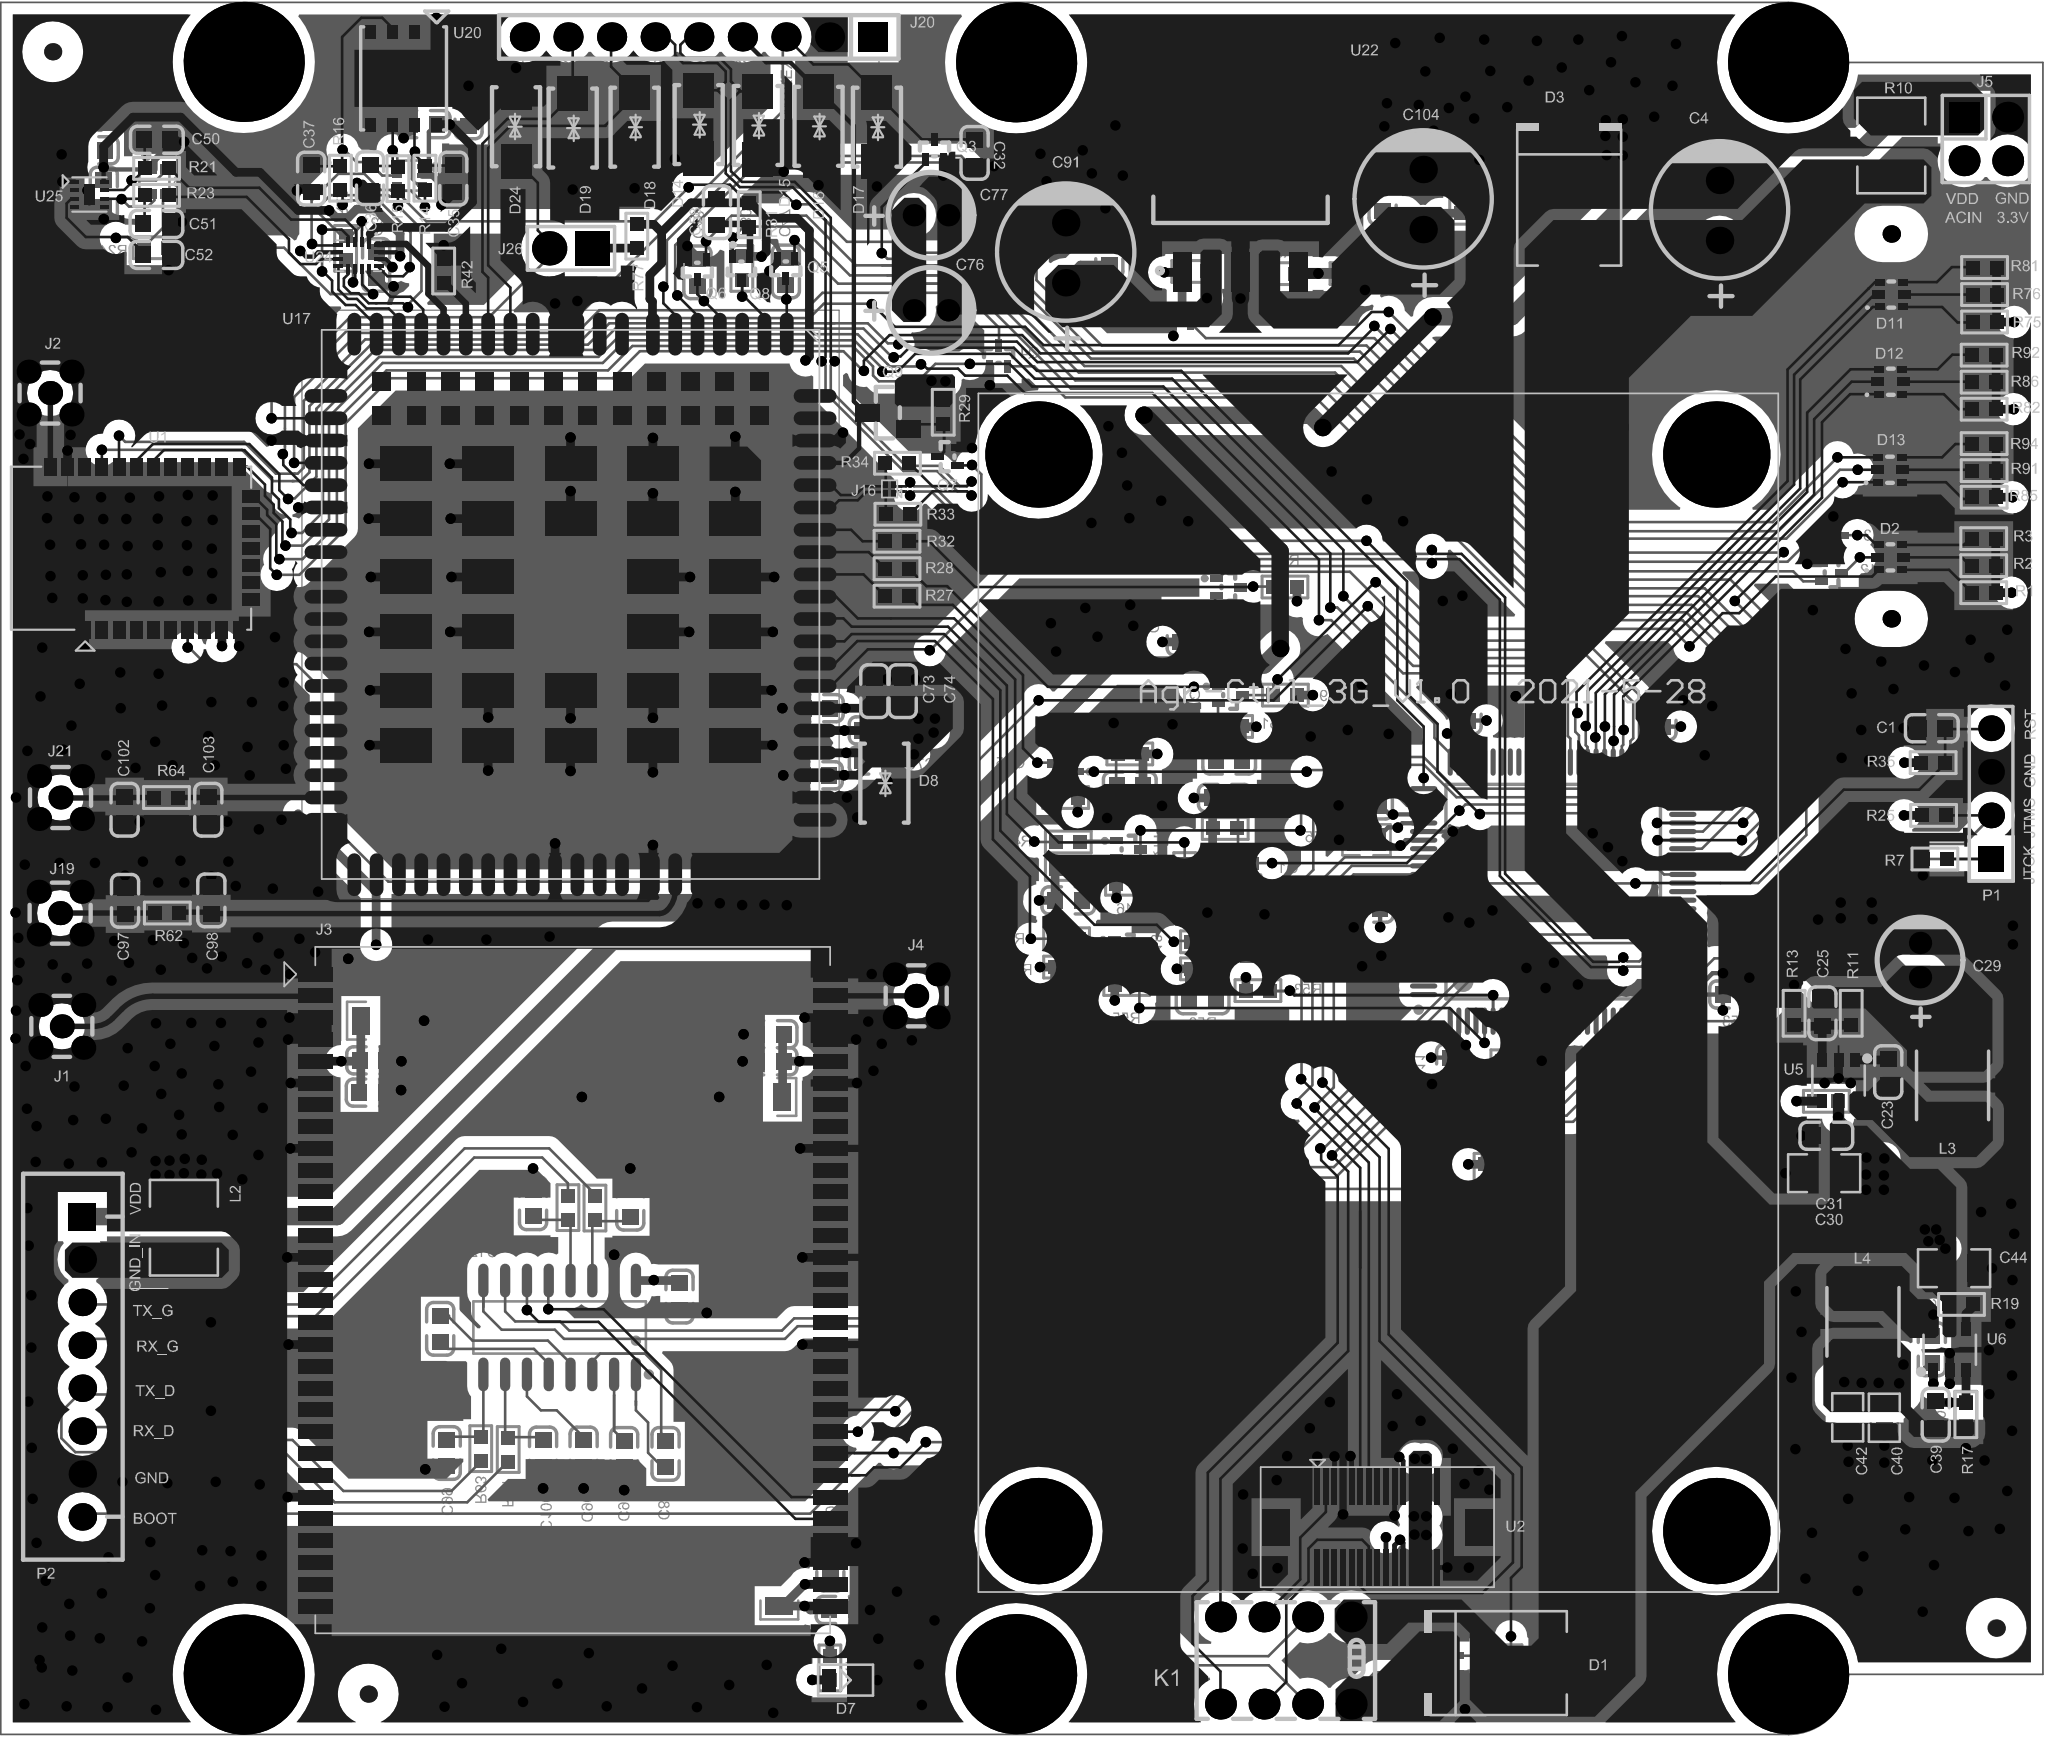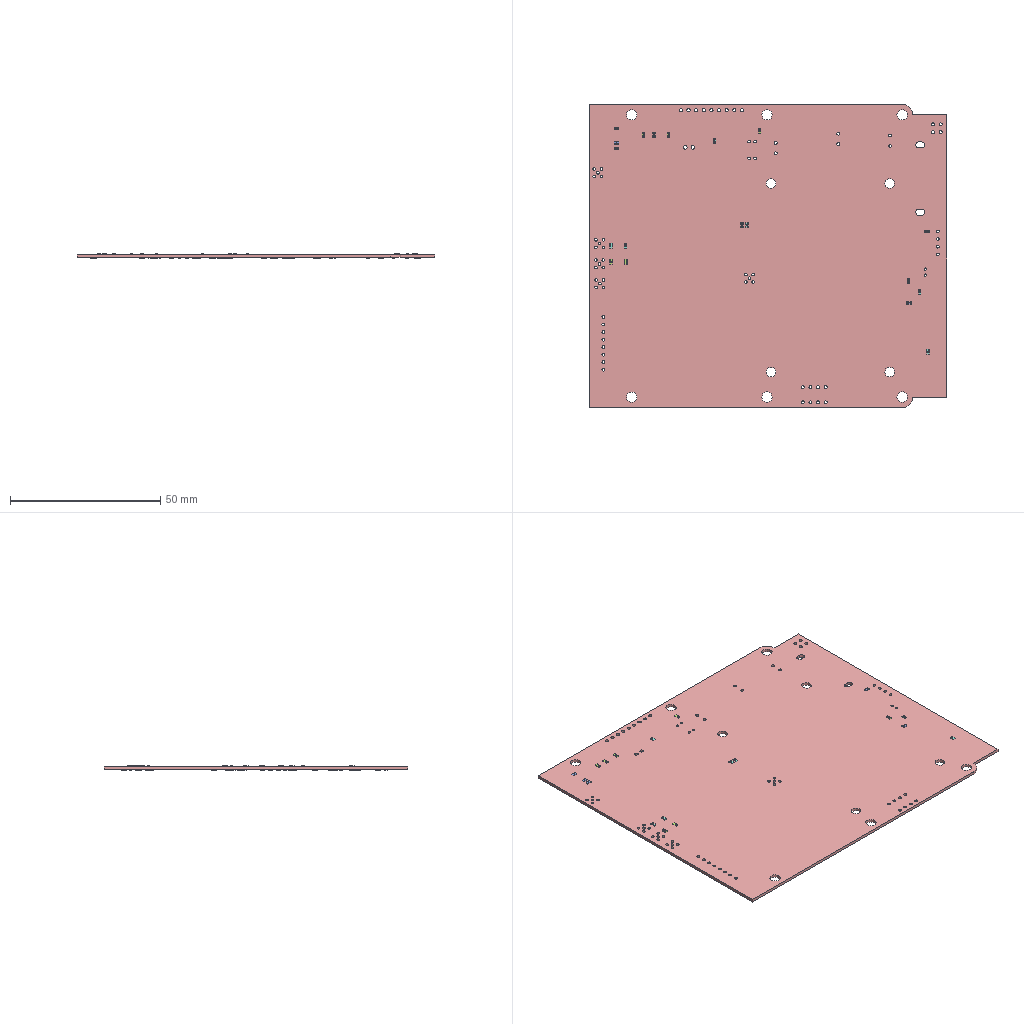Circuit board layout | Altium Designer | box 119 x 100.9 x 1.6 mm
Layer stack:
# Altium Designer layer stack of  (unit mm; dielectric type: 0 none, 1 core, 2 prepreg, 3 surface material)
index,name,kind,layer,copper_thickness_mm,dielectric_type,dielectric_thickness_mm,dielectric_material,dielectric_constant
0,Top Paste,other,,,,,,
1,Top Overlay,other,,,,,,
2,Top Solder,dielectric,,,3,0.0102,Solder Resist,3.5
3,TOP,copper,TOP,0.0305,,,,
4,Dielectric1,dielectric,,,1,0.2032,FR-4,4.5
5,GND,copper,GND,0.0356,,,,
6,Dielectric5,dielectric,,,2,0.32,FR-4,4.8
7,POWER,copper,POWER,0.0356,,,,
8,Dielectric6,dielectric,,,1,0.32,FR-4,4.8
9,BOTTOM,copper,BOTTOM,0.0305,,,,
10,Bottom Solder,dielectric,,,3,0.0102,Solder Resist,3.5
11,Bottom Overlay,other,,,,,,
12,Bottom Paste,other,,,,,,
# drill layer pairs: low layer,high layer
drill_pair,TOP,BOTTOM
Part placement:
Designator,Comment,Layer,Footprint,Center-X(mm),Center-Y(mm),Rotation
Q19,2SC4617TLQ,BottomLayer,SOT-416F_L1.6-W0.8-P1.00-LS1.6-TR,23.546,-26.391,270
Q18,2SC4617TLQ,BottomLayer,SOT-416F_L1.6-W0.8-P1.00-LS1.6-TR,4.953,15.342,90
Q17,2SC4617TLQ,BottomLayer,SOT-416F_L1.6-W0.8-P1.00-LS1.6-TR,12.624,15.215,90
Q16,2SC4617TLQ,BottomLayer,SOT-416F_L1.6-W0.8-P1.00-LS1.6-TR,10.973,30.099,90
Q15,2SC4617TLQ,BottomLayer,SOT-416F_L1.6-W0.8-P1.00-LS1.6-TR,1.397,26.137,270
Q14,2SC4617TLQ,BottomLayer,SOT-416F_L1.6-W0.8-P1.00-LS1.6-TR,5.055,21.107,90
C1,100nF/50V,TopLayer,C0603,51.867,28.169,360
C2,100nF/50V,BottomLayer,C0603,24.816,29.388,90
C3,100nF/50V,BottomLayer,C0603,36.17,29.032,90
C4,470uF/25V,TopLayer,RB8*11.5,39.497,58.344,90
C5,10uF/25V±10%,BottomLayer,C1206,-16.408,6.68,0
C6,100nF/50V,BottomLayer,C0603,-15.802,8.757,180
C7,100pF,BottomLayer,C0603,-15.799,10.338,180
C8,100pF,BottomLayer,C0603,-38.989,6.934,180
C9,100nF/50V,BottomLayer,C0603,-38.964,8.814,180
C10,10uF/25V±10%,BottomLayer,C1206,-38.379,11.125,180
C11,100nF/50V,BottomLayer,C0603,23.8,8.204,270
C20,100pF,BottomLayer,C0603,-12.319,-20.574,270
C21,100nF/50V,BottomLayer,C0603,-11.608,-23.216,180
C22,10uF/25V±10%,BottomLayer,C1206,-15.291,-21.666,270
C23,100nF/50V,TopLayer,C0603,49.327,8.128,90
C24,100nF/50V,BottomLayer,C0603,-33.401,64.059,90
C25,100pF,TopLayer,C0603,45.491,11.557,270
C26,22uF/10V±20%,BottomLayer,C0805,48.616,15.189,90
C27,100nF/50V,BottomLayer,C0603,44.577,15.189,90
C28,22uF/10V±20%,BottomLayer,C0805,46.558,15.189,90
C29,100uF/10V,TopLayer,RB5*7,51.181,14.656,90
C30,10uF/25V±10%,TopLayer,C1206,45.593,2.235,360
C31,100nF/50V,TopLayer,C0603,45.72,4.42,360
C32,10nF/50V,TopLayer,C0603,-3.912,61.697,270
C33,100nF/50V,BottomLayer,C0603,51.867,-8.026,270
C34,33pF/50V,BottomLayer,C0603,-36.017,63.373,180
C35,33pF/50V,TopLayer,C0603,-34.29,60.198,270
C36,33pF/50V,TopLayer,C0603,-39.141,60.223,270
C37,33pF/50V,TopLayer,C0603,-42.57,60.198,270
C38,100nF/50V,BottomLayer,C0603,-38.786,55.169,90
C39,100pF,TopLayer,C0603,52.095,-11.836,90
C40,22uF/10V±20%,TopLayer,C0805,49.098,-12.014,270
C41,100nF/50V,BottomLayer,C0603,49.098,-11.963,270
C42,22uF/10V±20%,TopLayer,C0805,46.965,-11.989,270
C43,22uF/10V±20%,BottomLayer,C0805,46.965,-11.989,270
C44,10uF/25V±10%,TopLayer,C1206,53.162,-3.302,180
C45,100nF/50V,BottomLayer,C0603,-55.347,61.849,180
C46,100nF/50V,BottomLayer,C0603,52.883,-0.0254,180
C47,10nF/50V,BottomLayer,C0603,-14.91,54.788,90
C48,10nF/50V,BottomLayer,C0603,-20.066,54.737,90
C49,33pF/50V,BottomLayer,C0603,-54.653,59.323,270
C50,33pF/50V,TopLayer,C0603,-51.562,62.459,360
C51,33pF/50V,TopLayer,C0603,-51.587,57.556,360
C52,33pF/50V,TopLayer,C0603,-51.587,55.753,360
C53,100nF/50V,BottomLayer,C0603,40.462,12.649,360
C54,100nF/50V,BottomLayer,C0603,18.948,17.653,180
C55,10nF/50V,BottomLayer,C0805,18.923,21.666,360
C56,100nF/50V,BottomLayer,C0603,18.898,23.673,180
C57,1nF/50V,BottomLayer,C0603,10.668,24.105,360
C58,1nF/50V,TopLayer,C0603,-18.923,58.242,90
C61,1nF/50V,BottomLayer,C0603,1.549,18.136,180
C62,1nF/50V,BottomLayer,C0603,10.922,26.289,360
C70,100nF/50V,BottomLayer,C0603,-9.677,26.289,360
C71,33pF/50V,BottomLayer,C0603,-9.677,28.042,360
C72,12pF/50V,BottomLayer,C0603,-13.106,29.337,180
C73,100nF/50V,TopLayer,C0603,-9.754,30.328,90
C74,33pF/50V,TopLayer,C0603,-8.103,30.328,90
C75,12pF/50V,BottomLayer,C0603,-13.157,25.425,180
C76,100uF/10V,TopLayer,RB5*7,-6.452,52.527,360
C77,100uF/10V,TopLayer,RB5*7,-6.452,58.064,360
C91,470uF/25V,TopLayer,RB8*11.5,1.397,55.88,90
C97,NM,TopLayer,C0603,-53.416,18.11,270
C98,NM,TopLayer,C0603,-48.387,18.136,270
C101,100nF/50V,BottomLayer,C0603,3.937,55.931,90
C102,NM,TopLayer,C0603,-53.442,23.419,90
C103,NM,TopLayer,C0603,-48.565,23.419,90
C104,470uF/25V,TopLayer,RB8*11.5,22.225,58.979,90
C105,100nF/50V,BottomLayer,C0603,19.863,59.055,90
D1,SMCJ18A,TopLayer,SMC,26.619,-26.314,360
D2,RGB,TopLayer,RGB,49.454,38.125,180
D3,SMCJ18A,TopLayer,SMC,30.734,59.106,270
D7,GREEN,TopLayer,LED0805,-11.43,-27.305,360
D8,SMAJ6.8CA,TopLayer,SMA,-9.169,24.968,180
D11,RGB,TopLayer,RGB,49.505,53.442,180
D12,RGB,TopLayer,RGB,49.479,48.362,180
D13,RGB,TopLayer,RGB,49.428,43.231,180
D14,SMAJ6.8CA,TopLayer,SMA,-19.99,63.348,180
D15,SMAJ6.8CA,TopLayer,SMA,-16.535,63.297,180
D16,SMAJ6.8CA,TopLayer,SMA,-13.005,63.246,180
D17,SMAJ6.8CA,TopLayer,SMA,-9.601,63.195,180
D18,SMAJ6.8CA,TopLayer,SMA,-23.724,63.195,180
D19,SMAJ6.8CA,TopLayer,SMA,-27.33,63.144,180
D24,SMAJ6.8CA,TopLayer,SMA,-30.632,63.221,360
J3,UM482/K823,TopLayer,UM482/K823,-27.33,-4.572,360
J4,MMCX-KE RF connector,TopLayer,MMCX-KE,-7.315,12.573,0
J5,POWER,TopLayer,2.54mm_2x2,55.016,62.509,270
U20,SIM-A China Telecom eSIM,TopLayer,VQFN8,-37.186,66.04,270
U23,ESDA6V8V6-6,BottomLayer,SOT-563,-36.83,60.376,180
U24,FSA2567MPX,TopLayer,MLP-16,-39.802,55.702,180
U25,SIM-B China Mobile eSIM,TopLayer,DFN2*2-8,-55.491,59.272,0
U26,ESDA6V8V6-6,BottomLayer,SOT-563,-51.706,60.009,270
J16,DLM0NSN900HY2D,TopLayer,SMD_0.85x0.65mm,-8.865,42.113,180
J20,2.54_9,TopLayer,2.54-9P,-19.984,68.456,180
J21,MMCX-KE RF connector,TopLayer,MMCX-KE,-57.175,24.13,0
L2,120Ω ±25% @100MHz,TopLayer,1812,-49.987,-0.9398,90
L3,2.2uH/2A,TopLayer,SMD,4x4x2.6mm,53.075,7.354,90
L4,2.2uH/2A,TopLayer,SMD,4x4x2.6mm,47.854,-6.426,270
P1,Header 4,TopLayer,HDR1X4,55.321,24.359,90
P2,XH-8A,TopLayer,XH-8A,-55.905,-9.042,270
Q1,2SC4617TLQ,BottomLayer,SOT-416F_L1.6-W0.8-P1.00-LS1.6-TR,11.938,19.609,360
Q2,8550,BottomLayer,SOT-23,26.797,5.766,180
Q3,DTC043ZEBTL,TopLayer,SOT-416_L1.6-W0.8-P1.00-LS1.6-BR,-6.248,61.9,0
Q4,DTC043ZEBTL,BottomLayer,SOT-416_L1.6-W0.8-P1.00-LS1.6-BR,-2.515,49.86,180
Q5,DTC043ZEBTL,TopLayer,SOT-416_L1.6-W0.8-P1.00-LS1.6-BR,-14.913,54.972,180
Q6,DTC043ZEBTL,TopLayer,SOT-416_L1.6-W0.8-P1.00-LS1.6-BR,-20.069,54.896,180
Q7,DTC043ZEBTL,TopLayer,SOT-416_L1.6-W0.8-P1.00-LS1.6-BR,-5.486,43.993,90
Q8,2SC4617TLQ,TopLayer,SOT-416F_L1.6-W0.8-P1.00-LS1.6-TR,-17.501,54.966,180
Q9,SI2333CDS-T1-E3,TopLayer,SOT-23_L2.9-W1.3-P1.90-LS2.4-BR,-8.966,46.558,90
Q10,DTC043ZEBTL,BottomLayer,SOT-416_L1.6-W0.8-P1.00-LS1.6-BR,8.179,52.375,180
Q11,2SC4617TLQ,BottomLayer,SOT-416F_L1.6-W0.8-P1.00-LS1.6-TR,10.871,36.398,90
Q12,DTC043ZEBTL,BottomLayer,SOT-416_L1.6-W0.8-P1.00-LS1.6-BR,46.025,37.236,90
Q13,DTC043ZEBTL,BottomLayer,SOT-416_L1.6-W0.8-P1.00-LS1.6-BR,46.05,39.421,90
R1,1K5,TopLayer,R0603,54.889,36.068,180
R2,680R,TopLayer,R0603,54.889,37.643,180
R3,1K,TopLayer,R0603,54.889,39.218,180
R4,10K,BottomLayer,R0603,29.159,29.337,270
R7,10K,TopLayer,R0603,52.045,20.549,180
R10,12V/2A,TopLayer,R1812,49.505,62.128,90
R11,75K 1%,TopLayer,R0603,47.168,11.557,90
R12,100K,BottomLayer,R0603,45.72,6.426,360
R13,10K,TopLayer,R0603,43.84,11.557,270
R14,22R,TopLayer,R0603,-35.941,60.223,90
R15,22R,TopLayer,R0603,-37.516,60.198,90
R16,22R,TopLayer,R0603,-40.869,60.223,90
R17,100K,TopLayer,R0603,53.848,-11.836,270
R18,1K,BottomLayer,R0603,-12.344,-26.594,270
R19,100K,TopLayer,R0603,53.594,-5.41,180
R20,22.1K 1%,BottomLayer,R0603,53.848,-11.811,90
R21,22R,TopLayer,R0603,-51.579,60.796,180
R22,NM,BottomLayer,R0603,-40.564,56.134,270
R23,22R,TopLayer,R0603,-51.579,59.221,180
R24,22R,BottomLayer,R0603,-51.605,56.171,180
R25,10K,TopLayer,R0603,51.968,23.089,180
R26,0R,BottomLayer,R0603,8.331,19.583,90
R27,0R,TopLayer,R0603,-8.433,35.865,180
R28,0R,TopLayer,R0603,-8.433,37.465,180
R29,10K,TopLayer,R0603,-5.74,46.584,270
R30,4.7K,BottomLayer,R0603,-17.475,54.966,270
R31,4.7K,TopLayer,R0603,-17.043,58.09,270
R32,0R,TopLayer,R0603,-8.433,39.065,180
R33,NM,TopLayer,R0603,-8.382,40.64,180
R34,NM,TopLayer,R0603,-8.407,43.612,180
R35,10K,TopLayer,R0603,51.943,26.162,180
R36,10K,BottomLayer,R0603,27.508,8.788,180
R37,10K,BottomLayer,R0603,27.762,2.032,270
R38,10K,BottomLayer,R0603,25.832,2.057,90
R39,4.7K,BottomLayer,R0603,10.693,22.327,180
R40,4.7K,BottomLayer,R0603,10.109,33.96,270
R41,10K,BottomLayer,R0603,9.957,19.583,270
R42,NM,TopLayer,R0603,-34.849,54.813,270
R43,4.7K,BottomLayer,R0603,5.131,26.67,360
R44,10K,BottomLayer,R0603,14.173,36.398,180
R45,10K,BottomLayer,R0603,1.397,24.13,180
R46,10K,BottomLayer,R0603,5.055,19.075,180
R47,0R,BottomLayer,R0603,1.549,21.539,180
R48,4.7K,BottomLayer,R0603,1.549,19.939,360
R49,10K,BottomLayer,R0603,14.199,30.099,360
R50,0R,BottomLayer,R0603,9.423,15.723,180
R51,4.7K,BottomLayer,R0603,10.947,28.27,180
R52,0R,BottomLayer,R0603,1.448,15.9,180
R53,10K,BottomLayer,R0603,12.598,12.878,180
R54,4.7K,BottomLayer,R0603,9.423,14.148,360
R55,10K,BottomLayer,R0603,4.953,13.233,180
R56,4.7K,BottomLayer,R0603,1.448,14.249,360
R57,4.7K,BottomLayer,R0603,26.645,-25.883,360
R59,4.7Ω,±1%,BottomLayer,R0603,-26.035,0.2058,270
R60,4.7Ω,±1%,BottomLayer,R0603,-27.61,0.2312,270
R61,4.7Ω,±1%,BottomLayer,R0603,-31.09,-13.866,90
R62,0R,TopLayer,R0603,-50.952,17.399,180
R63,4.7Ω,±1%,BottomLayer,R0603,-32.69,-13.815,90
R64,0R,TopLayer,R0603,-51.003,24.13,180
R65,47K,BottomLayer,R0603,8.915,54.788,360
R66,100K,BottomLayer,R0603,18.136,54.661,360
R67,330R,BottomLayer,R0603,24.409,58.877,270
R68,47K,BottomLayer,R0603,14.072,54.661,360
R75,1K5,TopLayer,R0603,54.94,51.841,180
R76,680R,TopLayer,R0603,54.94,53.442,180
R77,4.7K,TopLayer,R0603,-23.597,56.845,270
R81,1K,TopLayer,R0603,54.94,55.016,180
R82,1K5,TopLayer,R0603,54.915,46.761,180
R85,1K5,TopLayer,R0603,54.915,41.631,180
R86,680R,TopLayer,R0603,54.915,48.336,180
R91,680R,TopLayer,R0603,54.915,43.18,180
R92,1K,TopLayer,R0603,54.915,49.911,180
R94,1K,TopLayer,R0603,54.915,44.755,180
U1,HLK-B40,TopLayer,HLK-B40,-51.918,38.659,90
U2,24-5046-030-600-829,TopLayer,HX-DU1006D,19.558,11.69,180
U5,SY8113B,TopLayer,TSOT-23-6,46.431,7.636,90
U6,SY8113B,TopLayer,TSOT-23-6,52.908,-8.052,270
U8,STM32F103VCT6,BottomLayer,LQFP-100_14x14x05P,29.803,18.647,90
U12,SP3232EEN,BottomLayer,SOP16-6.6,-28.092,-6.754,90
U13,PESD15VL2BT,BottomLayer,SOT-23,-50.724,-6.452,90
U14,PESD15VL2BT,BottomLayer,SOT-23,-50.724,-11.608,90
U22,MIC29302WU,TopLayer,TO-263-5,11.582,59.436,360
C59,1nF/50V,BottomLayer,C0603,8.103,33.96,90
C60,1nF/50V,BottomLayer,C0603,5.131,24.816,180
C63,1nF/50V,BottomLayer,C0603,9.373,12.319,180
C64,1nF/50V,BottomLayer,C0603,1.473,12.471,180
C87,100nF/50V,BottomLayer,C0603,-21.92,-14.122,270
C88,100nF/50V,BottomLayer,C0603,-21.107,-4.953,270
C92,100nF/50V,BottomLayer,C0603,-24.333,-14.122,270
C93,100nF/50V,BottomLayer,C0603,-35.052,-6.833,90
C94,12pF/50V,BottomLayer,C0603,-23.978,0.4598,270
C95,12pF/50V,BottomLayer,C0603,-29.642,0.4852,270
C96,100nF/50V,BottomLayer,C0603,-26.695,-14.097,270
C99,12pF/50V,BottomLayer,C0603,-34.671,-14.069,270
C100,12pF/50V,BottomLayer,C0603,-29.058,-14.094,270
U17,EC20,TopLayer,EC20,-27.457,35.382,270
J26,2.54-2,TopLayer,2.54mm-2P,-27.432,56.134,180
J1,MMCX-KE RF connector,TopLayer,MMCX-KE,-57.099,10.795,0
J19,MMCX-KE RF connector,TopLayer,MMCX-KE,-57.198,17.393,0
J2,MMCX-KE RF connector,TopLayer,MMCX-KE,-57.785,47.701,270
K1,12V DPDT,TopLayer,G6K-2P_D12,14.224,-26.162,180
Pad and via stacks:
# Altium Designer via and pad stacks of  (unit mm). Each distinct definition once, with the count of objects using it.
# via: kind,start_layer,end_layer,hole_mm,diameter_mm,mode(0 simple;1 top-mid-bottom;2 full stack),diameter_per_layer,count,example_net
# pad: kind,layer,hole_mm,hole_type(0 round;1 square;2 slot),plating,top_size,top_shape(1 round;2 rect;3 octagon;9 rounded rect),mid_size,bottom_size,mode,footprint,size_per_layer,count,example
pad,TOP,0,0,plated,0.762x0.762,2,0.762x0.762,0.762x0.762,0,R0603,,70,R19.1
pad,TOP,0,0,plated,0.93x0.98,2,0.93x0.98,0.93x0.98,0,C0603,,38,C1.2
pad,TOP,0,0,plated,2x1.8,2,2x1.8,2x1.8,0,SMA,,16,D24.1
pad,TOP,0,0,plated,0.55x0.4,2,0.55x0.4,0.55x0.4,0,RGB,,16,D12.1
pad,TOP,0,0,plated,0.7x0.5,2,0.7x0.5,0.7x0.5,0,RGB,,8,D12.3
pad,TOP,0,0,plated,0.4x0.7,2,0.4x0.7,0.4x0.7,0,SOT-416_L1.6-W0.8-P1.00-LS1.6-BR,,12,Q5.3
pad,TOP,0,0,plated,0.8x1.3,2,0.8x1.3,0.8x1.3,0,LED0805,,2,D7.2
pad,TOP,0,0,plated,1.3x0.8,2,1.3x0.8,1.3x0.8,0,C0805,,4,C40.1
pad,TOP,0,0,plated,1x1.6,2,1x1.6,1x1.6,0,C1206,,4,C30.2
pad,TOP,0,0,plated,0.8x0.532,2,0.8x0.532,0.8x0.532,0,TSOT-23-6,,12,U5.1
pad,TOP,0,0,plated,3.7x1.9,2,3.7x1.9,3.7x1.9,0,SMD,4x4x2.6mm,,4,L3.1
pad,TOP,0,0,unplated,1x1,1,1x1,1x1,0,,,3,MARK
pad,TOP,0,0,plated,2.5x0.8,1,2.5x0.8,2.5x0.8,0,EC20,,80,U17.1
pad,TOP,0,0,plated,3x2,2,3x2,3x2,0,EC20,,27,U17.85
pad,TOP,0,0,plated,2x1,2,2x1,2x1,0,EC20,,1,U17.108
pad,TOP,0,0,plated,1.1x1.1,2,1.1x1.1,1.1x1.1,0,EC20,,24,U17.117
pad,TOP,0,0,plated,2.286x1.069,2,2.286x1.069,2.286x1.069,0,TO-263-5,,5,U22.1
pad,TOP,0,0,plated,10.66x8.89,2,10.66x8.89,10.66x8.89,0,TO-263-5,,1,U22.6
pad,TOP,0,0,plated,1.407x3.499,2,1.407x3.499,1.407x3.499,0,R1812,,2,R10.2
pad,TOP,0,0,plated,1.4x1,2,1.4x1,1.4x1,0,SOT-23_L2.9-W1.3-P1.90-LS2.4-BR,,3,Q9.2
pad,TOP,0,0,plated,0.4x0.7,2,0.4x0.7,0.4x0.7,0,SOT-416F_L1.6-W0.8-P1.00-LS1.6-TR,,2,Q8.2
pad,TOP,0,0,plated,0.5x0.7,2,0.5x0.7,0.5x0.7,0,SOT-416F_L1.6-W0.8-P1.00-LS1.6-TR,,1,Q8.3
pad,TOP,0,0,plated,1.407x3.499,2,1.407x3.499,1.407x3.499,0,1812,,2,L2.2
pad,TOP,0,0,plated,0.25x0.35,2,0.25x0.35,0.25x0.35,0,SMD_0.85x0.65mm,,4,J16.1
pad,TOP,0,0,plated,0.6x1.2,2,0.6x1.2,0.6x1.2,0,DFN2*2-8,,1,U25.9
pad,TOP,0,0,plated,0.2x0.5,2,0.2x0.5,0.2x0.5,0,DFN2*2-8,,8,U25.1
pad,TOP,0,0,plated,0.56x0.23,2,0.56x0.23,0.56x0.23,0,MLP-16,,15,U24.13
pad,TOP,0,0,plated,0.66x0.23,2,0.66x0.23,0.66x0.23,0,MLP-16,,1,U24.1
pad,TOP,0,0,plated,3.3x3.9,2,3.3x3.9,3.3x3.9,0,VQFN8,,1,U20.9
pad,TOP,0,0,plated,0.8x0.6,2,0.8x0.6,0.8x0.6,0,VQFN8,,8,U20.8
pad,TOP,0,0,plated,2.01x0.85,2,2.01x0.85,2.01x0.85,0,UM482/K823,,60,J3.60
pad,TOP,0,0,plated,2.158x3.24,2,2.158x3.24,2.158x3.24,0,SMC,,4,D3.1
pad,TOP,0,0,plated,2.1x1.6,2,2.1x1.6,2.1x1.6,0,HX-DU1006D,,2,U2.31
pad,TOP,0,0,plated,2.1x0.3,2,2.1x0.3,2.1x0.3,0,HX-DU1006D,,30,U2.2
pad,TOP,0,0,unplated,1x0.7,2,1x0.7,1x0.7,0,HLK-B40,,29,U1.2
pad,Multi-Layer,2,2,unplated,1.016x1.016,1,1.016x1.016,1.016x1.016,0,,,2,0
pad,Multi-Layer,3.5,0,plated,7x7,1,7x7,7x7,0,,,6,0
pad,Multi-Layer,1,0,plated,1.6x1.6,1,1.6x1.6,1.6x1.6,0,RB8*11.5,,6,C91.2
pad,Multi-Layer,0.9,0,plated,1.4x1.4,1,1.4x1.4,1.4x1.4,0,MMCX-KE,,25,J21.1
pad,Multi-Layer,0.8,0,plated,1.3x1.3,1,1.3x1.3,1.3x1.3,0,RB5*7,,6,C76.2
pad,Multi-Layer,1.2,0,plated,2x2,2,2x2,2x2,0,2.54mm-2P,,1,J26.1
pad,Multi-Layer,1.2,0,plated,2x2,1,2x2,2x2,0,2.54mm-2P,,1,J26.2
pad,Multi-Layer,1,0,plated,1.6x1.6,2,1.6x1.6,1.6x1.6,0,XH-8A,,1,P2.1
pad,Multi-Layer,1,0,plated,1.6x1.6,1,1.6x1.6,1.6x1.6,0,XH-8A,,7,P2.2
pad,Multi-Layer,1.1,0,plated,1.7x1.7,1,1.7x1.7,1.7x1.7,0,2.54-9P,,8,J20.9
pad,Multi-Layer,1.1,0,plated,1.7x1.7,2,1.7x1.7,1.7x1.7,0,2.54-9P,,1,J20.1
pad,Multi-Layer,1.05,0,plated,1.8x1.8,2,1.8x1.8,1.8x1.8,0,2.54mm_2x2,,1,J5.1
pad,Multi-Layer,1.05,0,plated,1.8x1.8,1,1.8x1.8,1.8x1.8,0,2.54mm_2x2,,3,J5.2
pad,Multi-Layer,0.9,0,plated,1.5x1.5,2,1.5x1.5,1.5x1.5,0,HDR1X4,,1,P1.1
pad,Multi-Layer,0.9,0,plated,1.5x1.5,1,1.5x1.5,1.5x1.5,0,HDR1X4,,3,P1.2
pad,Multi-Layer,1,0,plated,1.8x1.8,1,1.8x1.8,1.8x1.8,0,G6K-2P D12,,8,K1.8
pad,Multi-Layer,3.2,0,plated,6.2x6.2,1,6.2x6.2,6.2x6.2,0,HX-DU1006D,,4,U2.2
pad,BOTTOM,0,0,plated,0.762x0.762,2,0.762x0.762,0.762x0.762,0,R0603,,74,R12.1
pad,BOTTOM,0,0,plated,0.93x0.98,2,0.93x0.98,0.93x0.98,0,C0603,,90,C27.1
pad,BOTTOM,0,0,plated,1.3x0.8,2,1.3x0.8,1.3x0.8,0,C0805,,8,C26.1
pad,BOTTOM,0,0,plated,0.8x1,2,0.8x1,0.8x1,0,SOT-23,,9,U13.2
pad,BOTTOM,0,0,plated,0.602x1.971,1,0.602x1.971,0.602x1.971,0,SOP16-6.6,,16,U12.1
pad,BOTTOM,0,0,plated,0.4x0.7,2,0.4x0.7,0.4x0.7,0,SOT-416_L1.6-W0.8-P1.00-LS1.6-BR,,12,Q4.3
pad,BOTTOM,0,0,plated,1x1.6,2,1x1.6,1x1.6,0,C1206,,6,C5.2
pad,BOTTOM,0,0,plated,0.28x0.545,2,0.28x0.545,0.28x0.545,0,SOT-563,,12,U23.6
pad,BOTTOM,0,0,unplated,1x1,1,1x1,1x1,0,,,3,MARK
pad,BOTTOM,0,0,plated,0.5x0.7,2,0.5x0.7,0.5x0.7,0,SOT-416F_L1.6-W0.8-P1.00-LS1.6-TR,,8,Q19.3
pad,BOTTOM,0,0,plated,0.4x0.7,2,0.4x0.7,0.4x0.7,0,SOT-416F_L1.6-W0.8-P1.00-LS1.6-TR,,16,Q19.1
pad,BOTTOM,0,0,plated,0.3x1.6,1,0.3x1.6,0.3x1.6,0,LQFP-100_14x14x05P,,50,U8.1
pad,BOTTOM,0,0,plated,1.6x0.3,1,1.6x0.3,1.6x0.3,0,LQFP-100_14x14x05P,,50,U8.26
via,TOP,BOTTOM,0.3048,0.6096,0,,788,GND
via,TOP,BOTTOM,0.508,1.016,0,,4,VDD_IN
Copper pours:
name,layer,net,type(0 solid;1 hatched;2 none)
BottomLayer-No Net,TOP,VBAT,0
BottomLayer-No Net,TOP,VDD_12V,0
BottomLayer-No Net,TOP,VBAT,0
BottomLayer-No Net,TOP,VDD_12V,0
BottomLayer-No Net,TOP,VDD_5V,0
BottomLayer-No Net,TOP,GND_IN,0
BottomLayer-No Net,TOP,VDD_3V3,0
BottomLayer-No Net,TOP,VDD_5V,0
BottomLayer-No Net,TOP,NetD1_1,0
BottomLayer-No Net,TOP,NetC33_1,0
BottomLayer-No Net,TOP,VDD_3V3,0
BottomLayer-No Net,TOP,VDD_12V,0
BottomLayer-No Net,TOP,NetC23_1,0
BottomLayer-No Net,TOP,VDD_IN,0
BottomLayer-No Net,TOP,VDD_5V,0
BottomLayer-No Net,TOP,GND,0
BottomLayer-No Net,TOP,VBAT,0
BottomLayer-No Net,BOTTOM,GND,0
BottomLayer-No Net,BOTTOM,VDD_5V,0
BottomLayer-No Net,BOTTOM,VDD_3V3,0
Design rules, without the lines most boards share:
# Altium Designer design rules of  (exported by Altium Designer, unit mm)
# columns: name | kind | enabled | priority | scope1 | scope2 | descriptor | typed fields (field=value)
Clearance | 0 | enabled | 3 | All | All | Clearance Constraint (Gap=6mil) (All),(All) | gap=0.1524
PlaneConnect | 6 | enabled | 1 | All | All | Power Plane Connect Rule(Direct Connect )(Expansion=20mil) (Conductor Width=10mil) (Air Gap=10mil) (Entries=4) (All) | relief_conductor_width=0.254 relief_entries=4 relief_expansion=0.508
PlaneClearance | 12 | enabled | 1 | All | All | Power Plane Clearance (Clearance =10mil) (All) | clearance=0.254
PolygonConnect | 20 | enabled | 1 | All | All | Polygon Connect Rule(Direct Connect )(Conductor Width=10mil) (Relief Angle=90 Angle) (Entries=4) (Air Gap Width=10mil) (All),(All) | connect_style(0=relief,1=direct,2=none)=1 relief_conductor_width=0.254 relief_entries=4
Width | 2 | enabled | 1 | All | All | Width Constraint (Min=6mil) (Max=40mil) (Preferred=6mil) (All) |
RoutingVias | 11 | enabled | 1 | All | All | Routing Via (MinHoleWidth=12mil) (MaxHoleWidth=12mil) (PreferredHoleWidth=12mil) (MinWidth=24mil) (MaxWidth=24mil) (PreferedWidth=24mil) (All) | via_min_hole=0.3048 via_max_hole=0.3048 via_preferred_diameter=0.6096 via_preferred_hole=0.3048
SolderMaskExpansion | 13 | enabled | 1 | All | All | Solder Mask Expansion (Expansion =4mil) (All) | expansion=0.1016
HoleSize | 42 | enabled | 1 | All | All | Hole Size Constraint (Min=1mil) (Max=500mil) (All) |
DiffPairsRouting | 51 | enabled | 1 | All | All | Differential Pairs Uncoupled Length using the Gap Constraints (Min=6mil) (Max=6mil) (Prefered=6mil)  and Width Constraints (Min=15mil) (Max=15mil) (Prefered=15mil) (All) |
HoleToHoleClearance | 52 | enabled | 1 | All | All | Hole To Hole Clearance (Gap=0mil) (All),(All) | gap=0
MinimumSolderMaskSliver | 53 | enabled | 1 | All | All | Minimum Solder Mask Sliver (Gap=0mil) (All),(All) |
SilkscreenOverComponentPads | 54 | enabled | 1 | IsPad | All | Silk To Solder Mask (Clearance=0mil) (IsPad),(All) |
SilkToSilkClearance | 55 | enabled | 1 | All | All | Silk to Silk (Clearance=0mil) (All),(All) |
Clearance_1 | 0 | enabled | 2 | inpolygon | All | Clearance Constraint (Gap=6mil) (inpolygon),(All) | gap=0.1524
Clearance_2 | 0 | enabled | 1 | haspad('free-MARK') | All | Clearance Constraint (Gap=50mil) (haspad('free-MARK')),(All) | gap=1.27
Classes set for this board:
# Altium Designer classes of  (member kind: 0 net, 1 component, 2 from-to, 3 pad, 4 layer, 5 differential pair, 6 design channel, 7 polygon, 8 structure, 9 xSignal)
# columns: class name | member kind | superclass | members
Agr-Radio-TR_v1.0 | 1 | no | C1; C2; C3; C4; C5; C6; C7; C8; C9; C10; C11; C20; C21; C22; C23; C24; C25; C26; C27; C28; C29; C30; C31; C32; C33; C34; C35; C36; C37; C38; C39; C40; C41; C42; C43; C44; C45; C46; C47; C48; C49; C50; C51; C52; C53; C54; C55; C56; C57; C58; C59; C60; C61; C62; C63; C64; C70; C71; C72; C73; C74; C75; C76; C77; C87; C88; C91; C92; C93; C94; C95; C96; C97; C98; C99; C100; C101; C102; C103; C104; C105; D1; D2; D3; D7; D8; D11; D12; D13; D14; D15; D16; D17; D18; D19; J1; J2; J3; J4; J5; U20; U23; U24; U25; U26; J16; J19; J20; J21; J26; L2; L3; L4; P2; P2; Q1; Q2; Q3; Q4; Q5; Q6; Q7; Q8; Q9; Q10; Q11; Q12; Q13; R1; R2; R3; R4; R7; R10; R11; R12; R13; R14; R15; R16; R17; R18; R19; R20; R21; R22; R23; R24; R25; R26; R27; R28; R29; R30; R31; R32; R33; R34; R35; R36; R37; R38; R39; R40; R41; R42; R43; R44; R45; R46; R47; R48; R49; R50; R51; R52; R53; R54; R55; R56; R57; R59; R60; R61; R62; R63; R64; R65; R66; R67; R68; R75; R77; U1; U2; U5; U6; U8; U12; U13; U14; P2; C92; C93; C99; C100; P1; Q10; Q12; Q13; U12; Q9; J4; J14; J16; J21; R76; R81; R82; R85; R86; R91; R92; R94; D24; U22; C1; C2; C3; C4; C5; C6; C7; C8; C9; C10; C11; C20; C21; C22; C23; C24; C25; C26; C27; C28; C29; C30; C31; C32; C33; C34; C35; C36; C37; C38; C39; C40; C41; C42; C43; C44; C45; C46; C47; C48; C49; C50; C51; C52; C53; C54; C55; C56; C57; C58; C61; C62; C70; C71; C72; C73; C74; C75; C76; C77; C91; C97; C98; C101; C102; C103; C104; C105; D1; D2; D3; D7; D8; D11; D12; D13; D14; D15; D16; D17; D18; D19; D24; J3; J4; J5; J10; J11; J12; J13; J14; J16; J20; J21; L2; L3; L4; P1; P2; Q1; Q2; Q3; Q4; Q5; Q6; Q7; Q8; Q9; Q10; Q11; Q12; Q13; R1; R2; R3; R4; R7; R10; R11; R12; R13; R14; R15; R16; R17; R18; R19; R20; R21; R22; R23; R24; R25; R26; R27; R28; R29; R30; R31; R32; R33; R34; R35; R36; R37; R38; R39; R40; R41; R42; R43; R44; R45; R46; R47; R48; R49; R50; R51; R52; R53; R54; R55; R56; R57; R59; R60; R61; R62; R63; R64; R65; R66; R67; R68; R75; R76; R77; R81; R82; R85; R86; R91; R92; R94; U1; U2; U5; U6; U8; U12; U13; U14; U22; C59; C60; C63; C64; C87; C88; C92; C93; C94; C95; C96; C99; C100; U17; J26; J1; J19; J2; Q14; Q15; Q16; Q17; Q18; Q19; K1;